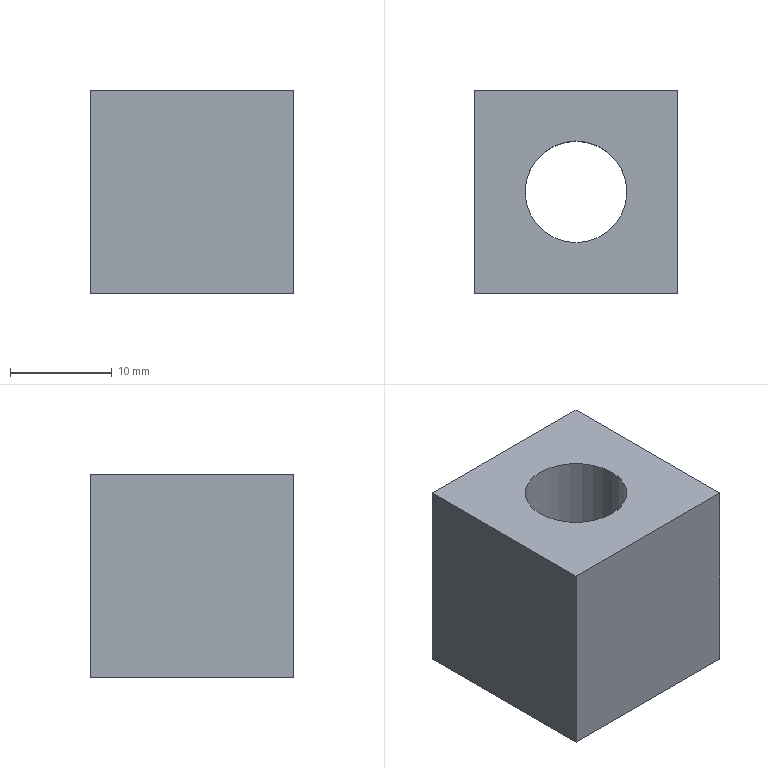Part | SolidWorks | features Cut 1, Extrusion 1 | 1 solid | 8 faces | box 20 x 20 x 20 mm | volume 6429 mm3 | plane 6 | cylinder 2 | commonest cylinder face diameters 10 x2
STEP:
#1=CARTESIAN_POINT('',(-5.,0.,0.));
#2=VERTEX_POINT('',#1);
#3=CARTESIAN_POINT('',(5.,0.,0.));
#4=VERTEX_POINT('',#3);
#5=CARTESIAN_POINT('',(0.,0.,0.));
#6=DIRECTION('',(0.,0.,1.));
#7=DIRECTION('',(1.,0.,0.));
#8=AXIS2_PLACEMENT_3D('',#5,#6,#7);
#9=CIRCLE('',#8,5.);
#10=EDGE_CURVE('',#2,#4,#9,.T.);
#11=ORIENTED_EDGE('',*,*,#10,.F.);
#12=CARTESIAN_POINT('',(-5.,0.,20.));
#13=VERTEX_POINT('',#12);
#14=CARTESIAN_POINT('',(-5.,0.,0.));
#15=DIRECTION('',(0.,0.,1.));
#16=VECTOR('',#15,1000.);
#17=LINE('',#14,#16);
#18=EDGE_CURVE('',#2,#13,#17,.T.);
#19=ORIENTED_EDGE('',*,*,#18,.T.);
#20=CARTESIAN_POINT('',(5.,0.,20.));
#21=VERTEX_POINT('',#20);
#22=CARTESIAN_POINT('',(0.,0.,20.));
#23=DIRECTION('',(0.,0.,1.));
#24=DIRECTION('',(1.,0.,0.));
#25=AXIS2_PLACEMENT_3D('',#22,#23,#24);
#26=CIRCLE('',#25,5.);
#27=EDGE_CURVE('',#13,#21,#26,.T.);
#28=ORIENTED_EDGE('',*,*,#27,.T.);
#29=CARTESIAN_POINT('',(5.,0.,0.));
#30=DIRECTION('',(0.,0.,1.));
#31=VECTOR('',#30,1000.);
#32=LINE('',#29,#31);
#33=EDGE_CURVE('',#4,#21,#32,.T.);
#34=ORIENTED_EDGE('',*,*,#33,.F.);
#35=EDGE_LOOP('',(#11,#19,#28,#34));
#36=FACE_OUTER_BOUND('',#35,.T.);
#37=CARTESIAN_POINT('',(0.,0.,0.));
#38=DIRECTION('',(0.,0.,1.));
#39=DIRECTION('',(1.,0.,0.));
#40=AXIS2_PLACEMENT_3D('',#37,#38,#39);
#41=CYLINDRICAL_SURFACE('',#40,5.);
#42=ADVANCED_FACE('',(#36),#41,.F.);
#43=CARTESIAN_POINT('',(10.,-10.,0.));
#44=VERTEX_POINT('',#43);
#45=CARTESIAN_POINT('',(10.,10.,0.));
#46=VERTEX_POINT('',#45);
#47=CARTESIAN_POINT('',(10.,-10.,0.));
#48=DIRECTION('',(0.,1.,0.));
#49=VECTOR('',#48,1000.);
#50=LINE('',#47,#49);
#51=EDGE_CURVE('',#44,#46,#50,.T.);
#52=ORIENTED_EDGE('',*,*,#51,.T.);
#53=CARTESIAN_POINT('',(10.,10.,20.));
#54=VERTEX_POINT('',#53);
#55=CARTESIAN_POINT('',(10.,10.,20.));
#56=DIRECTION('',(0.,0.,-1.));
#57=VECTOR('',#56,1000.);
#58=LINE('',#55,#57);
#59=EDGE_CURVE('',#54,#46,#58,.T.);
#60=ORIENTED_EDGE('',*,*,#59,.F.);
#61=CARTESIAN_POINT('',(10.,-10.,20.));
#62=VERTEX_POINT('',#61);
#63=CARTESIAN_POINT('',(10.,-10.,20.));
#64=DIRECTION('',(0.,1.,0.));
#65=VECTOR('',#64,1000.);
#66=LINE('',#63,#65);
#67=EDGE_CURVE('',#62,#54,#66,.T.);
#68=ORIENTED_EDGE('',*,*,#67,.F.);
#69=CARTESIAN_POINT('',(10.,-10.,20.));
#70=DIRECTION('',(0.,0.,-1.));
#71=VECTOR('',#70,1000.);
#72=LINE('',#69,#71);
#73=EDGE_CURVE('',#62,#44,#72,.T.);
#74=ORIENTED_EDGE('',*,*,#73,.T.);
#75=EDGE_LOOP('',(#52,#60,#68,#74));
#76=FACE_OUTER_BOUND('',#75,.T.);
#77=CARTESIAN_POINT('',(10.,-10.,20.));
#78=DIRECTION('',(-1.,0.,0.));
#79=DIRECTION('',(0.,-1.,0.));
#80=AXIS2_PLACEMENT_3D('',#77,#78,#79);
#81=PLANE('',#80);
#82=ADVANCED_FACE('',(#76),#81,.F.);
#83=CARTESIAN_POINT('',(-10.,10.,0.));
#84=VERTEX_POINT('',#83);
#85=CARTESIAN_POINT('',(10.,10.,0.));
#86=DIRECTION('',(-1.,0.,0.));
#87=VECTOR('',#86,1000.);
#88=LINE('',#85,#87);
#89=EDGE_CURVE('',#46,#84,#88,.T.);
#90=ORIENTED_EDGE('',*,*,#89,.T.);
#91=CARTESIAN_POINT('',(-10.,10.,20.));
#92=VERTEX_POINT('',#91);
#93=CARTESIAN_POINT('',(-10.,10.,20.));
#94=DIRECTION('',(0.,0.,-1.));
#95=VECTOR('',#94,1000.);
#96=LINE('',#93,#95);
#97=EDGE_CURVE('',#92,#84,#96,.T.);
#98=ORIENTED_EDGE('',*,*,#97,.F.);
#99=CARTESIAN_POINT('',(10.,10.,20.));
#100=DIRECTION('',(-1.,0.,0.));
#101=VECTOR('',#100,1000.);
#102=LINE('',#99,#101);
#103=EDGE_CURVE('',#54,#92,#102,.T.);
#104=ORIENTED_EDGE('',*,*,#103,.F.);
#105=ORIENTED_EDGE('',*,*,#59,.T.);
#106=EDGE_LOOP('',(#90,#98,#104,#105));
#107=FACE_OUTER_BOUND('',#106,.T.);
#108=CARTESIAN_POINT('',(10.,10.,20.));
#109=DIRECTION('',(0.,-1.,0.));
#110=DIRECTION('',(1.,0.,0.));
#111=AXIS2_PLACEMENT_3D('',#108,#109,#110);
#112=PLANE('',#111);
#113=ADVANCED_FACE('',(#107),#112,.F.);
#114=CARTESIAN_POINT('',(-10.,-10.,0.));
#115=VERTEX_POINT('',#114);
#116=CARTESIAN_POINT('',(-10.,10.,0.));
#117=DIRECTION('',(0.,-1.,0.));
#118=VECTOR('',#117,1000.);
#119=LINE('',#116,#118);
#120=EDGE_CURVE('',#84,#115,#119,.T.);
#121=ORIENTED_EDGE('',*,*,#120,.T.);
#122=CARTESIAN_POINT('',(-10.,-10.,20.));
#123=VERTEX_POINT('',#122);
#124=CARTESIAN_POINT('',(-10.,-10.,20.));
#125=DIRECTION('',(0.,0.,-1.));
#126=VECTOR('',#125,1000.);
#127=LINE('',#124,#126);
#128=EDGE_CURVE('',#123,#115,#127,.T.);
#129=ORIENTED_EDGE('',*,*,#128,.F.);
#130=CARTESIAN_POINT('',(-10.,10.,20.));
#131=DIRECTION('',(0.,-1.,0.));
#132=VECTOR('',#131,1000.);
#133=LINE('',#130,#132);
#134=EDGE_CURVE('',#92,#123,#133,.T.);
#135=ORIENTED_EDGE('',*,*,#134,.F.);
#136=ORIENTED_EDGE('',*,*,#97,.T.);
#137=EDGE_LOOP('',(#121,#129,#135,#136));
#138=FACE_OUTER_BOUND('',#137,.T.);
#139=CARTESIAN_POINT('',(-10.,10.,20.));
#140=DIRECTION('',(1.,0.,0.));
#141=DIRECTION('',(0.,1.,0.));
#142=AXIS2_PLACEMENT_3D('',#139,#140,#141);
#143=PLANE('',#142);
#144=ADVANCED_FACE('',(#138),#143,.F.);
#145=CARTESIAN_POINT('',(-10.,-10.,0.));
#146=DIRECTION('',(1.,0.,0.));
#147=VECTOR('',#146,1000.);
#148=LINE('',#145,#147);
#149=EDGE_CURVE('',#115,#44,#148,.T.);
#150=ORIENTED_EDGE('',*,*,#149,.T.);
#151=ORIENTED_EDGE('',*,*,#73,.F.);
#152=CARTESIAN_POINT('',(-10.,-10.,20.));
#153=DIRECTION('',(1.,0.,0.));
#154=VECTOR('',#153,1000.);
#155=LINE('',#152,#154);
#156=EDGE_CURVE('',#123,#62,#155,.T.);
#157=ORIENTED_EDGE('',*,*,#156,.F.);
#158=ORIENTED_EDGE('',*,*,#128,.T.);
#159=EDGE_LOOP('',(#150,#151,#157,#158));
#160=FACE_OUTER_BOUND('',#159,.T.);
#161=CARTESIAN_POINT('',(-10.,-10.,20.));
#162=DIRECTION('',(0.,1.,0.));
#163=DIRECTION('',(-1.,0.,0.));
#164=AXIS2_PLACEMENT_3D('',#161,#162,#163);
#165=PLANE('',#164);
#166=ADVANCED_FACE('',(#160),#165,.F.);
#167=CARTESIAN_POINT('',(0.,0.,20.));
#168=DIRECTION('',(0.,0.,1.));
#169=DIRECTION('',(1.,0.,0.));
#170=AXIS2_PLACEMENT_3D('',#167,#168,#169);
#171=CIRCLE('',#170,5.);
#172=EDGE_CURVE('',#21,#13,#171,.T.);
#173=ORIENTED_EDGE('',*,*,#172,.F.);
#174=ORIENTED_EDGE('',*,*,#27,.F.);
#175=EDGE_LOOP('',(#173,#174));
#176=FACE_BOUND('',#175,.T.);
#177=ORIENTED_EDGE('',*,*,#67,.T.);
#178=ORIENTED_EDGE('',*,*,#103,.T.);
#179=ORIENTED_EDGE('',*,*,#134,.T.);
#180=ORIENTED_EDGE('',*,*,#156,.T.);
#181=EDGE_LOOP('',(#177,#178,#179,#180));
#182=FACE_OUTER_BOUND('',#181,.T.);
#183=CARTESIAN_POINT('',(10.,-10.,20.));
#184=DIRECTION('',(0.,0.,-1.));
#185=DIRECTION('',(-1.,0.,0.));
#186=AXIS2_PLACEMENT_3D('',#183,#184,#185);
#187=PLANE('',#186);
#188=ADVANCED_FACE('',(#176,#182),#187,.F.);
#189=CARTESIAN_POINT('',(0.,0.,0.));
#190=DIRECTION('',(0.,0.,1.));
#191=DIRECTION('',(1.,0.,0.));
#192=AXIS2_PLACEMENT_3D('',#189,#190,#191);
#193=CIRCLE('',#192,5.);
#194=EDGE_CURVE('',#4,#2,#193,.T.);
#195=ORIENTED_EDGE('',*,*,#194,.T.);
#196=ORIENTED_EDGE('',*,*,#10,.T.);
#197=EDGE_LOOP('',(#195,#196));
#198=FACE_BOUND('',#197,.T.);
#199=ORIENTED_EDGE('',*,*,#51,.F.);
#200=ORIENTED_EDGE('',*,*,#149,.F.);
#201=ORIENTED_EDGE('',*,*,#120,.F.);
#202=ORIENTED_EDGE('',*,*,#89,.F.);
#203=EDGE_LOOP('',(#199,#200,#201,#202));
#204=FACE_OUTER_BOUND('',#203,.T.);
#205=CARTESIAN_POINT('',(10.,-10.,0.));
#206=DIRECTION('',(0.,0.,-1.));
#207=DIRECTION('',(-1.,0.,0.));
#208=AXIS2_PLACEMENT_3D('',#205,#206,#207);
#209=PLANE('',#208);
#210=ADVANCED_FACE('',(#198,#204),#209,.T.);
#211=ORIENTED_EDGE('',*,*,#18,.F.);
#212=ORIENTED_EDGE('',*,*,#194,.F.);
#213=ORIENTED_EDGE('',*,*,#33,.T.);
#214=ORIENTED_EDGE('',*,*,#172,.T.);
#215=EDGE_LOOP('',(#211,#212,#213,#214));
#216=FACE_OUTER_BOUND('',#215,.T.);
#217=CARTESIAN_POINT('',(0.,0.,0.));
#218=DIRECTION('',(0.,0.,1.));
#219=DIRECTION('',(1.,0.,0.));
#220=AXIS2_PLACEMENT_3D('',#217,#218,#219);
#221=CYLINDRICAL_SURFACE('',#220,5.);
#222=ADVANCED_FACE('',(#216),#221,.F.);
#223=CLOSED_SHELL('',(#42,#82,#113,#144,#166,#188,#210,#222));
#224=MANIFOLD_SOLID_BREP('',#223);
#225=CARTESIAN_POINT('',(0.,0.,0.));
#226=DIRECTION('',(0.,0.,1.));
#227=DIRECTION('',(1.,0.,0.));
#228=AXIS2_PLACEMENT_3D('',#225,#226,#227);
#229=(LENGTH_UNIT()NAMED_UNIT(*)SI_UNIT(.MILLI.,.METRE.));
#230=UNCERTAINTY_MEASURE_WITH_UNIT(LENGTH_MEASURE(0.00001),#229,'','');
#231=(NAMED_UNIT(*)PLANE_ANGLE_UNIT()SI_UNIT($,.RADIAN.));
#232=(NAMED_UNIT(*)SI_UNIT($,.STERADIAN.)SOLID_ANGLE_UNIT());
#233=(GEOMETRIC_REPRESENTATION_CONTEXT(3)GLOBAL_UNCERTAINTY_ASSIGNED_CONTEXT((#230))GLOBAL_UNIT_ASSIGNED_CONTEXT((#229,#231,#232))REPRESENTATION_CONTEXT('',''));
#234=ADVANCED_BREP_SHAPE_REPRESENTATION('',(#224,#228),#233);